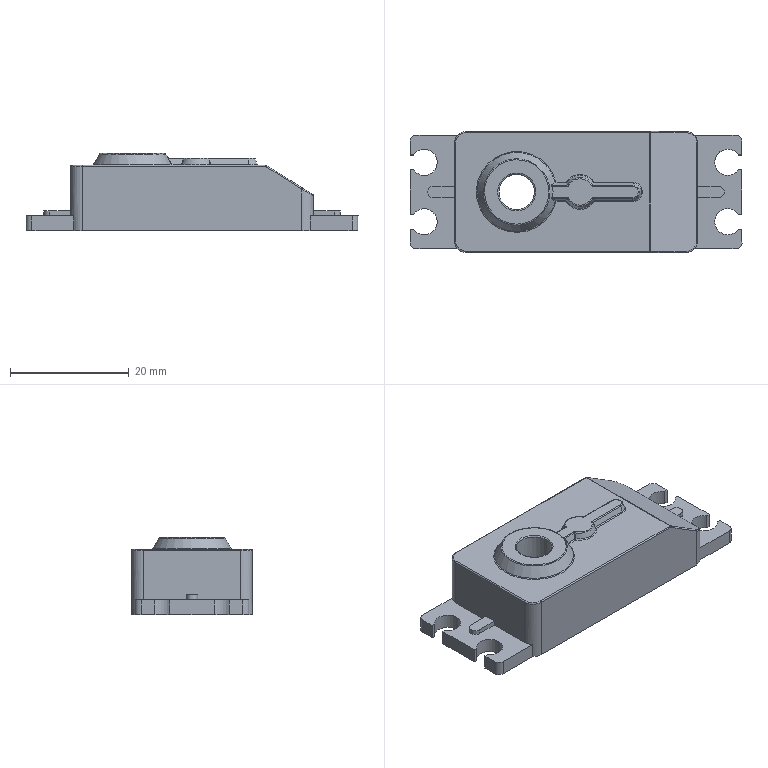Part | STEP file | Zapas-OpenRC Truggy HSPr v2. v55-2 | 1 solid | 116 faces | box 56 x 20.4 x 13 mm | volume 9258 mm3 | plane 41 | cylinder 35 | spline 33 | cone 4 | sphere 3 | commonest cylinder face diameters 0.4 x15 2 x7 4.4 x6 4 x4 1.4 x2 6 x1